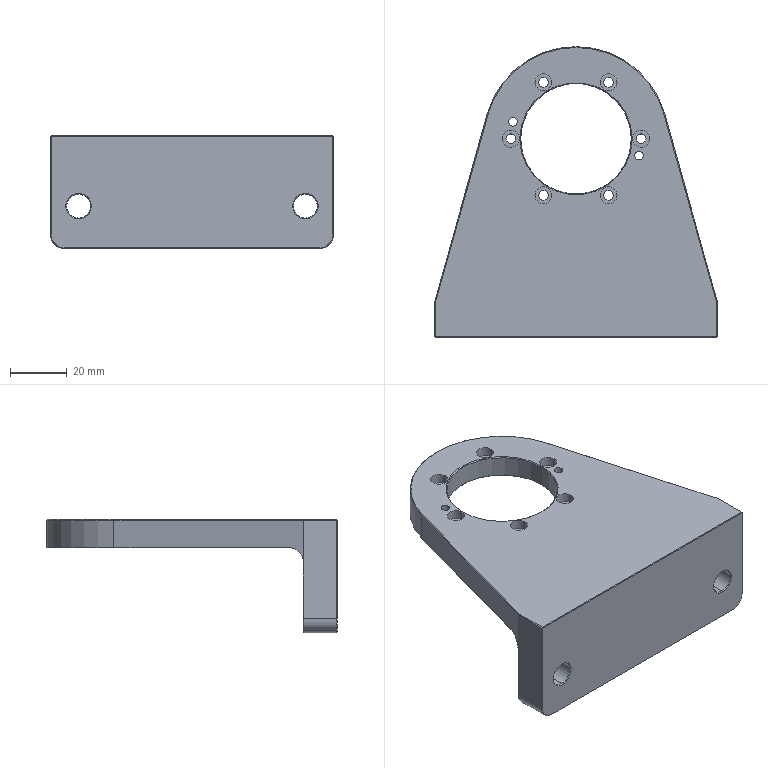NC program | NX | posted with a generic post | part box 100 x 102.5 x 40 mm
Lines 70 to 995 of 4503:
(ADAPTIVE_MILLING , TOOL : D10)
N120 T15 M6
N122 G54
N124 G17 G0 G90 X-39.298 Y62.694 B0. C0. S9500 M3
N126 G43 Z30. H15
N128 Z-17.
N130 G94 G1 Z-20. F1000.
N132 X-39.828 Y61.338 F3000.
N134 G3 X-39.298 Y60.047 R1.015
N136 X-36.138 Y59.404 R9.424
N138 X-24.642 Y59.208 R185.073
N140 G1 X-19.242 Y59.206
N142 X53.458
N144 X53.658 Y59.203
N146 X53.758 Y59.199
N148 X53.858 Y59.193
N150 X53.957 Y59.185
N152 G2 X58.292 Y56.274 R6.04
N154 X60.077 Y50.703 R13.203
N156 X60.422 Y42.315 R76.732
N158 G1 X60.429 Y40.915
N160 X60.434 Y39.015
N162 X60.437 Y35.815
N164 X60.439 Y26.715
N166 Y-52.285
N168 X60.437 Y-52.385
N170 G2 X57.938 Y-56.743 R5.754
N172 X52.455 Y-58.757 R12.082
N174 X43.972 Y-59.169 R66.869
N176 G1 X42.672 Y-59.177
N178 X40.972 Y-59.182
N180 X38.272 Y-59.186
N182 X32.672 Y-59.188
N184 X-53.528
N186 X-53.628 Y-59.187
N188 G2 X-58.106 Y-56.528 R5.815
N190 X-60.033 Y-51.012 R12.428
N192 X-60.423 Y-42.126 R73.754
N194 G1 X-60.43 Y-40.626
N196 X-60.435 Y-38.426
N198 X-60.438 Y-34.626
N200 X-60.439 Y-17.626
N202 Y38.974
N204 X-60.442 Y39.974
N206 G2 X-60.42 Y52.773 R766.33
N208 X-57.54 Y57.022 R6.066
N210 X-52.074 Y58.811 R13.054
N212 X-43.887 Y59.171 R72.631
N214 X-38.005 Y58.794 R42.391
N216 G3 X-25.915 Y58.424 R142.287
N218 G1 X-23.615 Y58.419
N220 X-20.015 Y58.415
N222 X-10.015 Y58.414
N224 X50.785
N226 X50.985 Y58.41
N228 X51.185 Y58.402
N230 G2 X57.273 Y54.557 R7.641
N232 X59.221 Y48.304 R15.498
N234 X59.615 Y38.417 R90.294
N236 G1 X59.621 Y36.817
N238 X59.626 Y34.517
N240 X59.629 Y30.617
N242 X59.63 Y15.917
N244 Y-49.483
N246 X59.628 Y-49.683
N248 G2 X55.908 Y-55.943 R7.565
N250 X49.776 Y-57.938 R15.014
N252 X40.191 Y-58.361 R82.486
N254 G1 X38.691 Y-58.369
N256 X36.691 Y-58.374
N258 X33.491 Y-58.378
N260 X26.091 Y-58.38
N262 X-50.709
N264 X-50.909 Y-58.378
N266 G2 X-57.18 Y-54.677 R7.557
N268 X-59.212 Y-48.35 R15.239
N270 X-59.609 Y-39.264 R82.815
N272 G1 X-59.617 Y-37.864
N274 X-59.623 Y-35.964
N276 X-59.627 Y-33.264
N278 X-59.63 Y-27.964
N280 Y36.236
N282 X-59.636 Y37.436
N284 G2 X-59.615 Y50.235 R604.146
N286 X-55.617 Y56.128 R7.75
N288 X-49.138 Y58.02 R16.241
N290 X-38.357 Y58.002 R55.026
N292 G3 X-21.565 Y57.627 R248.66
N294 G1 X-17.565 Y57.624
N296 X-6.765 Y57.623
N298 X48.135 Y57.622
N300 X48.435 Y57.62
N302 X48.635 Y57.618
N304 X48.835 Y57.613
N306 G2 X56.511 Y52.825 R8.831
N308 X58.428 Y46.037 R18.036
N310 X58.808 Y35.049 R112.657
N312 G1 X58.814 Y33.049
N314 X58.819 Y30.149
N316 X58.821 Y24.649
N318 X58.822 Y-20.951
N320 X58.825 Y-21.951
N322 X58.827 Y-23.551
N324 X58.826 Y-25.051
N326 X58.828 Y-25.951
N328 Y-26.851
N330 X58.83 Y-27.951
N332 X58.829 Y-28.951
N334 X58.83 Y-29.851
N336 X58.829 Y-30.851
N338 X58.831 Y-31.751
N340 X58.829 Y-32.651
N342 X58.831 Y-33.651
N344 X58.829 Y-34.751
N346 X58.831 Y-35.751
N348 X58.829 Y-36.851
N350 X58.83 Y-37.651
N352 X58.829 Y-38.651
N354 X58.831 Y-39.651
N356 X58.829 Y-40.651
N358 G2 X58.786 Y-48.25 R212.358
N360 X53.982 Y-55.292 R8.813
N362 X47.187 Y-57.185 R18.173
N364 X35.898 Y-57.56 R117.998
N366 G1 X33.898 Y-57.565
N368 X30.798 Y-57.569
N370 X24.198 Y-57.571
N372 X-48.402
N374 X-48.602 Y-57.569
N376 X-48.802 Y-57.565
N378 G2 X-56.545 Y-52.727 R8.81
N380 X-58.454 Y-45.732 R18.397
N382 X-58.811 Y-34.242 R126.498
N384 G1 X-58.817 Y-31.942
N386 X-58.82 Y-28.242
N388 X-58.821 Y-18.442
N390 X-58.822 Y33.458
N392 X-58.828 Y34.758
N394 X-58.83 Y36.258
N396 G2 X-58.807 Y48.157 R460.428
N398 X-54.076 Y55.248 R8.808
N400 X-47.192 Y57.185 R17.971
N402 X-39.101 Y57.212 R49.816
N404 G3 X-21.208 Y56.838 R325.602
N406 G1 X-17.808 Y56.834
N408 X-11.308 Y56.832
N410 X45.492 Y56.831
N412 X46.192 Y56.827
N414 X46.492 Y56.824
N416 X46.692 Y56.82
N418 G2 X55.822 Y51.112 R9.789
N420 X57.619 Y44.18 R20.375
N422 X57.999 Y32.69 R124.75
N424 G1 X58.005 Y30.69
N426 X58.01 Y27.79
N428 X58.012 Y22.49
N430 X58.013 Y-18.21
N432 X58.018 Y-19.31
N434 X58.02 Y-20.81
N436 Y-22.41
N438 X58.023 Y-23.31
N440 X58.024 Y-24.61
N442 X58.027 Y-25.51
N444 X58.026 Y-26.81
N446 X58.028 Y-27.61
N448 Y-28.81
N450 X58.029 Y-29.71
N452 X58.028 Y-30.61
N454 X58.03 Y-31.51
N456 X58.029 Y-32.51
N458 X58.031 Y-33.51
N460 X58.029 Y-34.61
N462 X58.03 Y-35.61
N464 X58.029 Y-36.41
N466 X58.031 Y-37.41
N468 X58.029 Y-38.51
N470 G2 X57.965 Y-46.608 R162.791
N472 X52.621 Y-54.424 R9.634
N474 X45.424 Y-56.366 R19.82
N476 X34.635 Y-56.745 R117.504
N478 G1 X32.835 Y-56.753
N480 X30.435 Y-56.758
N482 X26.835 Y-56.761
N484 X16.835 Y-56.762
N486 X-46.365
N488 X-46.565 Y-56.761
N490 G2 X-53.076 Y-54.646 R10.034
N492 G1 X-53.461 Y-54.486
N494 X-53.58 Y-54.418
N496 G2 X-55.736 Y-52.211 R7.144
N498 X-57.708 Y-43.572 R25.584
N500 X-58.005 Y-30.979 R182.312
N502 G1 X-58.009 Y-28.179
N504 X-58.012 Y-23.179
N506 X-58.013 Y11.221
N508 Y30.721
N510 X-58.017 Y31.621
N512 X-58.019 Y32.621
N514 G2 X-58.015 Y46.121 R784.268
N516 X-55.877 Y51.873 R9.634
N518 G1 X-55.736 Y52.211
N520 X-55.668 Y52.33
N522 G2 X-53.461 Y54.486 R7.144
N524 X-43.717 Y56.433 R24.504
N526 X-32.621 Y56.164 R346.097
N528 G3 X-12.522 Y56.041 R869.916
N530 G1 X8.478 Y56.04
N532 X42.778
N534 X43.978 Y56.033
N536 X44.478 Y56.029
N538 X44.978 Y56.02
N540 X45.178 Y56.015
N542 G2 X52.192 Y53.546 R10.616
N544 X56.022 Y46.996 R13.055
N546 X57.066 Y38.578 R38.218
N548 X57.203 Y22.18 R583.22
N550 G1 X57.204 Y7.78
N552 X57.205 Y-15.52
N554 X57.209 Y-16.42
N556 X57.211 Y-17.62
N558 X57.215 Y-18.42
N560 Y-18.92
N562 X57.214 Y-19.82
N564 X57.219 Y-20.92
N566 Y-22.02
N568 X57.222 Y-23.02
N570 Y-24.22
N572 X57.225 Y-25.22
N574 X57.224 Y-26.22
N576 X57.227 Y-27.22
N578 X57.226 Y-28.42
N580 X57.228 Y-29.32
N582 X57.227 Y-30.62
N584 X57.229 Y-31.42
N586 X57.228 Y-32.42
N588 X57.23 Y-33.52
N590 X57.229 Y-34.32
N592 X57.231 Y-35.42
N594 X57.229 Y-36.32
N596 G2 X57.165 Y-44.919 R201.547
N598 X51.289 Y-53.601 R10.297
N600 X43.784 Y-55.555 R21.276
N602 X31.795 Y-55.94 R134.94
N604 G1 X29.695 Y-55.946
N606 X26.695 Y-55.951
N608 X21.195 Y-55.953
N610 X-44.305 Y-55.954
N612 X-44.705 Y-55.952
N614 X-45.005 Y-55.948
N616 G2 X-49.614 Y-55.155 R14.255
N618 X-52.346 Y-54.948 R11.744
N620 G1 X-53.086 Y-54.642
N622 X-53.337 Y-54.539
N624 X-53.58 Y-54.418
N626 G2 X-55.736 Y-52.211 R7.227
N628 G1 X-56.198 Y-51.096
N630 G2 X-56.516 Y-47.77 R31.1
N632 X-57.185 Y-32.292 R148.725
N634 G1 X-57.192 Y-30.492
N636 X-57.199 Y-27.992
N638 X-57.202 Y-24.292
N640 X-57.204 Y-15.992
N642 X-57.205 Y28.008
N644 X-57.209 Y28.908
N646 G2 X-57.199 Y44.608 R764.429
N648 X-56.408 Y48.411 R13.691
N650 X-56.198 Y51.096 R11.906
N652 G1 X-55.854 Y51.928
N654 G3 X-57.97 Y52.356 R-1.1
N656 G1 X-58.6 Y-49.559
N658 G3 X-57.505 Y-50.664 R1.1
N660 X-56.4 Y-49.566 R1.1
N662 G1 Y48.534
N664 G2 X-56.198 Y51.096 R10.617
N666 X-54.564 Y53.663 R6.015
N668 G1 X-53.58 Y54.418
N670 X-53.461 Y54.486
N672 X-52.346 Y54.948
N674 G2 X-49.418 Y55.227 R22.217
N676 X-38.63 Y55.519 R79.437
N678 G3 X-10.533 Y55.249 R913.498
N680 G1 X16.567
N682 X40.067 Y55.248
N684 X41.867 Y55.237
N686 X42.667 Y55.232
N688 X43.167 Y55.225
N690 G2 X49.086 Y54.007 R13.093
N692 X54.523 Y47.721 R11.639
N694 X56.075 Y40.107 R26.204
N696 X56.387 Y26.913 R190.336
N698 G1 X56.392 Y24.013
N700 X56.395 Y19.113
N702 X56.396 Y-2.987
N704 Y-12.787
N706 X56.4 Y-13.687
N708 X56.402 Y-14.987
N710 X56.407 Y-15.987
N712 X56.408 Y-17.387
N714 X56.413 Y-18.487
N716 Y-19.587
N718 X56.417 Y-20.687
N720 Y-21.687
N722 X56.421 Y-22.787
N724 Y-23.887
N726 X56.424 Y-24.887
N728 X56.423 Y-26.087
N730 X56.426 Y-27.087
N732 X56.425 Y-28.187
N734 X56.428 Y-29.187
N736 X56.426 Y-30.287
N738 X56.428 Y-31.187
N740 Y-32.487
N742 G2 X56.36 Y-43.385 R285.575
N744 X49.959 Y-52.819 R10.87
N746 X42.437 Y-54.727 R22.416
N748 X30.249 Y-55.13 R135.397
N750 G1 X28.349 Y-55.136
N752 X25.649 Y-55.141
N754 X21.149 Y-55.144
N756 X6.249 Y-55.145
N758 X-39.182
N760 X-39.232 Y-55.149
N762 X-39.268 Y-55.15
N764 X-49.668
N766 G3 X-50.592 Y-55.767 R1.01
N768 G1 X-51.385 Y-57.603 Z-19.9
N770 G2 X-51.778 Y-58.218 R1.418
N772 X-52.85 Y-58.332 R1.011
N774 G1 X-53.966 Y-57.774
N776 X-55.058 Y-57.168
N778 G2 X-56.726 Y-55.945 R10.968
N780 X-57.789 Y-54.689 R7.418
N782 X-58.716 Y-53.097 R9.68
N784 X-59.266 Y-50.733 R6.939
N786 X-59.511 Y-43.244 R172.458
N788 G1 X-60.256 Y43.234
N790 G2 X-59.232 Y51.387 R31.064
N792 G1 X-58.921 Y52.574
N794 X-58.592 Y53.757
N796 G2 X-56.392 Y56.398 R4.86
N798 G1 X-54.613 Y57.4
N800 G2 X-53.424 Y57.246 R1.009
N802 G1 X-51.939 Y55.907 Z-20.
N804 X-51.27 Y55.317
N806 G3 X-50.716 Y55.15 R1.05
N808 G1 X-39.268
N810 X-39.232 Y55.149
N812 G2 X-36.033 Y54.791 R234.525
N814 G3 X-21.739 Y54.475 R237.987
N816 G1 X-19.239 Y54.467
N818 X-15.939 Y54.462
N820 X-10.939 Y54.458
N822 X2.561 Y54.457
N824 X37.361
N826 X39.061 Y54.447
N828 G2 X44.65 Y54.202 R39.414
N830 X53.145 Y47.774 R11.258
N832 X55.146 Y39.968 R22.992
N834 X55.565 Y28.48 R125.908
N836 G1 X55.573 Y26.78
N838 X55.579 Y24.68
N840 X55.584 Y21.38
N842 X55.586 Y15.68
N844 X55.587 Y7.68
N846 X55.594 Y7.581
N848 X55.597 Y7.557
N850 X55.805 Y6.657
N852 X55.815 Y6.605
N854 X56.29 Y2.855
N856 X56.294 Y2.801
N858 X56.386 Y-0.992
N860 X56.385 Y-1.025
N862 G2 X55.821 Y-6.734 R65.3
N864 G3 X55.619 Y-15.629 R121.735
N866 G1 Y-17.829
N868 X55.622 Y-20.029
N870 X55.623 Y-20.529
N872 X55.621 Y-21.329
N874 X55.622 Y-21.929
N876 X55.623 Y-22.529
N878 X55.622 Y-23.529
N880 X55.625 Y-24.729
N882 X55.623 Y-25.829
N884 X55.626 Y-26.829
N886 X55.625 Y-27.829
N888 X55.627 Y-28.929
N890 X55.626 Y-29.929
N892 X55.628 Y-30.929
N894 X55.627 Y-32.029
N896 G2 X55.549 Y-42.028 R228.856
N898 X48.958 Y-51.907 R11.314
N900 X41.251 Y-53.892 R22.815
N902 X29.863 Y-54.313 R124.104
N904 G1 X28.263 Y-54.322
N906 X26.163 Y-54.328
N908 X23.263 Y-54.333
N910 X18.163 Y-54.336
N912 X-4.937 Y-54.337
N914 X-35.537
N916 G2 X-38.514 Y-55.095 R179.175
N918 G1 X-38.585 Y-55.104
N920 X-39.183 Y-55.145
N922 G3 X-39.181 Y-57.141 R1.
N924 G1 X-38.933 Y-57.157
N926 X-36.938 Y-57.289 Z-19.9
N928 X-35.286 Y-57.395
N930 X37.839
N932 G3 X44.014 Y-56.718 R28.808
N934 G1 X45.354 Y-56.418
N936 X46.682 Y-56.07
N938 G3 X52.578 Y-53.178 R19.723
N940 X54.882 Y-51.398 R24.071
N942 X56.148 Y-49.792 R7.044
N944 X57.478 Y-47.115 R26.695
N946 X58.16 Y-44.598 R12.677
N948 X58.554 Y-40.889 R22.015
N950 G1 X59.159 Y-8.626
N952 X59.139 Y-8.427
N954 X59.088 Y-8.234
N956 X58.358 Y-6.418
N958 X58.099 Y-5.764 Z-19.935
N960 X57.824 Y-5.117 Z-19.97
N962 G3 X57.394 Y-4.721 Z-20. R1.049
N964 X55.977 Y-5.444 R1.003
N966 X55.089 Y-10.498 R100.777
N968 X54.84 Y-18.691 R94.439
N970 G1 X54.832 Y-21.191
N972 X54.827 Y-23.691
N974 X54.826 Y-26.191
N976 X54.829 Y-28.691
N978 X54.83 Y-29.291
N980 X54.828 Y-29.991
N982 X54.829 Y-30.791
N984 X54.83 Y-31.391
N986 X54.829 Y-32.291
N988 X54.83 Y-33.091
N990 X54.829 Y-33.891
N992 X54.83 Y-34.891
N994 G2 X54.662 Y-41.585 R71.054
N996 X47.791 Y-51.102 R11.67
N998 X40.075 Y-53.06 R23.64
N1000 X28.588 Y-53.502 R121.257
N1002 G1 X26.988 Y-53.511
N1004 X24.888 Y-53.518
N1006 X22.088 Y-53.524
N1008 X17.588 Y-53.527
N1010 X4.788 Y-53.528
N1012 X-32.612
N1014 X-32.712 Y-53.533
N1016 X-32.819 Y-53.547
N1018 X-35.804 Y-54.383
N1020 G3 X-35.987 Y-56.237 R1.001
N1022 X-35.33 Y-56.365 Z-19.966 R1.675
N1024 G1 X-34.009 Y-56.47 Z-19.9
N1026 X-31.907 Y-56.633
N1028 X33.093
N1030 G3 X41.798 Y-55.96 R59.876
N1032 X48.961 Y-53.908 R26.424
N1034 X53.588 Y-50.782 R18.657
N1036 X55.048 Y-49.258 R11.046
N1038 X56.633 Y-46.172 R11.229
N1040 X57.627 Y-41.314 R16.524
N1042 G1 X57.787 Y-38.823
N1044 X57.892 Y-36.329
N1046 X58.58 Y-11.806
N1048 X58.559 Y-11.593
N1050 X58.501 Y-11.388
N1052 X57.739 Y-9.591
N1054 X57.481 Y-8.972 Z-19.934
N1056 X57.203 Y-8.363 Z-19.967
N1058 G3 X56.697 Y-7.958 Z-20. R1.041
N1060 X55.398 Y-8.624 R1.004
N1062 X54.378 Y-12.795 R25.967
N1064 X54.055 Y-20.985 R80.133
N1066 G1 X54.047 Y-22.385
N1068 X54.041 Y-24.085
N1070 X54.039 Y-26.085
N1072 X54.038 Y-26.685
N1074 X54.034 Y-27.485
N1076 Y-28.285
N1078 X54.035 Y-28.885
N1080 X54.032 Y-29.785
N1082 Y-30.585
N1084 Y-31.085
N1086 X54.031 Y-31.885
N1088 X54.032 Y-32.885
N1090 X54.027 Y-34.285
N1092 Y-34.985
N1094 X54.024 Y-35.785
N1096 X54.015 Y-36.885
N1098 G2 X53.363 Y-42.828 R21.168
N1100 X46.799 Y-50.231 R11.995
N1102 X38.891 Y-52.243 R24.374
N1104 X26.904 Y-52.694 R127.347
N1106 G1 X25.204 Y-52.703
N1108 X23.004 Y-52.71
N1110 X20.004 Y-52.715
N1112 X15.004 Y-52.718
N1114 X-1.696 Y-52.72
N1116 X-29.696
N1118 X-29.796 Y-52.722
N1120 X-29.895 Y-52.732
N1122 X-29.934 Y-52.738
N1124 X-32.823 Y-53.548
N1126 G3 X-33.006 Y-55.402 R1.001
N1128 X-32.349 Y-55.53 Z-19.966 R1.675
N1130 G1 X-31.028 Y-55.635 Z-19.9
N1132 X-28.926 Y-55.798
N1134 X34.199
N1136 G3 X41.014 Y-55.127 R35.788
N1138 X47.599 Y-53.244 R34.595
N1140 X51.331 Y-51.033 R15.261
N1142 G1 X52.025 Y-50.413
N1144 X52.68 Y-49.751
N1146 X53.481 Y-48.876
N1148 X54.269 Y-47.989
N1150 G3 X55.694 Y-45.397 R8.933
N1152 G1 X55.921 Y-44.688
N1154 X56.109 Y-43.967
N1156 G3 X56.8 Y-40.293 R39.084
N1158 G1 X56.925 Y-39.055
N1160 X57.002 Y-37.812
N1162 X57.864 Y-14.306
N1164 X57.844 Y-14.088
N1166 X57.785 Y-13.878
N1168 X57.025 Y-12.092
N1170 X56.766 Y-11.472 Z-19.934
N1172 X56.487 Y-10.862 Z-19.967
N1174 G3 X55.983 Y-10.459 Z-20. R1.041
N1176 X54.682 Y-11.124 R1.004
N1178 G2 X53.929 Y-13.453 R66.85
N1180 G3 X53.325 Y-19.713 R31.007
N1182 X53.201 Y-36.512 R978.881
N1184 G2 X52.221 Y-42.701 R17.893
N1186 X45.342 Y-49.589 R12.517
N1188 X37.294 Y-51.469 R26.261
N1190 X25.305 Y-51.886 R141.796
N1192 G1 X23.505 Y-51.895
N1194 X21.205 Y-51.902
N1196 X18.005 Y-51.907
N1198 X12.805 Y-51.91
N1200 X-6.895 Y-51.911
N1202 X-26.795
N1204 X-26.895 Y-51.912
N1206 X-26.994 Y-51.921
N1208 X-27.05 Y-51.93
N1210 X-29.938 Y-52.74
N1212 G3 X-30.122 Y-54.594 R1.001
N1214 X-29.465 Y-54.722 Z-19.966 R1.675
N1216 G1 X-28.144 Y-54.826 Z-19.9
N1218 X-26.041 Y-54.99
N1220 X32.709
N1222 G3 X40.136 Y-54.254 R38.314
N1224 G1 X42.705 Y-53.726
N1226 G3 X49.38 Y-50.748 R20.14
N1228 X51.755 Y-48.931 R19.855
N1230 X53.42 Y-46.918 R11.577
N1232 X55.442 Y-42.423 R13.539
N1234 X55.947 Y-39.358 R19.463
N1236 G1 X56.173 Y-36.872
N1238 X56.341 Y-34.381
N1240 X57.315 Y-15.966
N1242 X57.296 Y-15.729
N1244 X57.227 Y-15.5
N1246 X56.447 Y-13.781
N1248 X56.18 Y-13.18 Z-19.933
N1250 X55.89 Y-12.589 Z-19.966
N1252 G3 X55.349 Y-12.193 Z-20. R1.039
N1254 X54.133 Y-12.784 R1.005
N1256 X52.661 Y-19.172 R16.325
N1258 X52.44 Y-31.868 R253.297
N1260 G2 X52.188 Y-38.46 R59.193
N1262 X44.786 Y-48.548 R12.545
N1264 X36.78 Y-50.585 R25.095
N1266 X25.195 Y-51.068 R117.402
N1268 G1 X23.695 Y-51.079
N1270 X21.895 Y-51.087
N1272 X19.595 Y-51.094
N1274 X16.395 Y-51.098
N1276 X10.895 Y-51.101
N1278 X-11.005 Y-51.102
N1280 X-23.905
N1282 X-24.005 Y-51.103
N1284 X-24.105 Y-51.112
N1286 X-24.164 Y-51.122
N1288 X-27.053 Y-51.931
N1290 G3 X-27.236 Y-53.786 R1.001
N1292 X-26.579 Y-53.913 Z-19.966 R1.674
N1294 G1 X-25.258 Y-54.018 Z-19.9
N1296 X-23.156 Y-54.181
N1298 X30.594
N1300 G3 X38.043 Y-53.565 R45.87
N1302 G1 X39.707 Y-53.289
N1304 X41.362 Y-52.967
N1306 G3 X46.284 Y-51.224 R21.017
N1308 G1 X47.391 Y-50.613
N1310 X48.487 Y-49.982
N1312 G3 X51.373 Y-47.508 R13.567
N1314 X53.98 Y-43.3 R12.588
N1316 X55.129 Y-38.48 R16.719
N1318 G1 X55.376 Y-35.996
N1320 X55.573 Y-33.507
N1322 X56.617 Y-17.733
N1324 X56.6 Y-17.488
N1326 X56.529 Y-17.252
N1328 X55.751 Y-15.547
N1330 X55.483 Y-14.945 Z-19.933
N1332 X55.192 Y-14.355 Z-19.966
N1334 G3 X54.651 Y-13.96 Z-20. R1.039
N1336 X53.436 Y-14.551 R1.005
N1338 X52.516 Y-16.82 R49.659
N1340 X51.801 Y-22.563 R25.85
N1342 X51.596 Y-34.461 R772.828
N1344 G2 X50.476 Y-40.928 R18.353
N1346 X43.483 Y-47.859 R12.987
N1348 X35.149 Y-49.829 R27.118
N1350 X22.961 Y-50.266 R142.214
N1352 G1 X21.461 Y-50.274
N1354 X19.361 Y-50.282
N1356 X16.561 Y-50.288
N1358 X12.361 Y-50.292
N1360 X3.361 Y-50.294
N1362 X-21.039
N1364 X-21.139 Y-50.296
N1366 X-21.238 Y-50.307
N1368 X-21.275 Y-50.313
N1370 X-24.164 Y-51.122
N1372 G3 X-24.347 Y-52.976 R1.001
N1374 X-23.69 Y-53.104 Z-19.966 R1.674
N1376 G1 X-22.369 Y-53.209 Z-19.9
N1378 X-20.267 Y-53.372
N1380 X29.108
N1382 G3 X37.788 Y-52.589 R48.938
N1384 G1 X40.86 Y-52.018
N1386 G3 X44.369 Y-50.793 R17.143
N1388 X47.662 Y-49.018 R22.672
N1390 X50.515 Y-46.618 R18.947
N1392 X52.597 Y-43.833 R17.2
N1394 X53.637 Y-41.306 R12.099
N1396 X54.539 Y-35.779 R23.838
N1398 G1 X55.115 Y-19.782
N1400 X55.007 Y-18.621
N1402 X54.88 Y-17.463
N1404 X54.81 Y-16.773 Z-19.935
N1406 X54.722 Y-16.084 Z-19.969
N1408 G3 X54.4 Y-15.576 Z-20. R1.046
N1410 X52.865 Y-15.884 R1.003
N1412 X51.251 Y-21.092 R11.886
N1414 X50.876 Y-30.18 R102.783
N1416 G2 X50.514 Y-36.765 R51.24
N1418 X42.716 Y-46.936 R13.032
N1420 X34.302 Y-48.989 R26.84
N1422 X21.215 Y-49.46 R143.887
N1424 G1 X19.315 Y-49.469
N1426 X16.915 Y-49.476
N1428 X13.615 Y-49.481
N1430 X8.215 Y-49.484
N1432 X-9.885 Y-49.485
N1434 X-18.185
N1436 G3 X-21.276 Y-50.313 R31.257
N1438 X-21.459 Y-52.167 R1.001
N1440 X-20.802 Y-52.295 Z-19.966 R1.674
N1442 G1 X-19.481 Y-52.4 Z-19.9
N1444 X-17.379 Y-52.563
N1446 X25.121
N1448 G3 X35.083 Y-51.948 R82.023
N1450 G1 X38.8 Y-51.475
N1452 G3 X42.499 Y-50.404 R16.766
N1454 X45.202 Y-49.119 R27.7
N1456 G1 X46.218 Y-48.566
N1458 X47.208 Y-47.969
N1460 G3 X49.666 Y-45.807 R13.519
N1462 X52.253 Y-41.592 R11.977
N1464 X53.538 Y-36.474 R22.892
N1466 G1 X53.695 Y-35.081
N1468 X53.799 Y-33.683
N1470 X54.432 Y-21.117
N1472 X54.427 Y-20.961
N1474 X54.197 Y-18.799
N1476 X54.127 Y-18.108 Z-19.935
N1478 X54.039 Y-17.419 Z-19.97
N1480 G3 X53.717 Y-16.911 Z-20. R1.047
N1482 X52.182 Y-17.22 R1.003
N1484 X50.479 Y-22.608 R12.457
N1486 X50.072 Y-30.895 R104.762
N1488 G2 X49.406 Y-37.247 R29.345
N1490 X42.148 Y-45.925 R13.109
N1492 X33.971 Y-48.096 R25.482
N1494 X22.589 Y-48.63 R109.277
N1496 G1 X21.389 Y-48.641
N1498 X19.789 Y-48.652
N1500 X17.789 Y-48.661
N1502 X15.289 Y-48.668
N1504 X11.789 Y-48.673
N1506 X5.889 Y-48.676
N1508 X-15.311 Y-48.677
N1510 X-15.41 Y-48.683
N1512 X-15.509 Y-48.697
N1514 X-18.398 Y-49.507
N1516 G3 X-18.582 Y-51.361 R1.001
N1518 X-17.924 Y-51.489 Z-19.966 R1.674
N1520 G1 X-16.604 Y-51.593 Z-19.9
N1522 X-14.501 Y-51.757
N1524 X27.999
N1526 G3 X35.438 Y-51.086 R42.087
N1528 G1 X38.017 Y-50.604
N1530 G3 X45.549 Y-47.419 R21.783
N1532 X48.255 Y-45.417 R32.285
N1534 X50.414 Y-42.708 R10.137
N1536 X51.85 Y-39.535 R28.839
N1538 X52.661 Y-35.919 R15.2
N1540 X53.373 Y-27.205 R244.774
N1542 G1 X53.659 Y-22.542
N1544 X53.402 Y-20.287
N1546 X53.33 Y-19.62 Z-19.934
N1548 X53.235 Y-18.956 Z-19.967
N1550 G3 X52.866 Y-18.426 Z-20. R1.041
N1552 X51.407 Y-18.734 R1.004
N1554 X49.848 Y-22.959 R9.202
N1556 X49.298 Y-30.535 R72.328
N1558 G2 X48.414 Y-36.956 R25.749
N1560 X41.028 Y-45.184 R13.394
N1562 X32.733 Y-47.307 R26.42
N1564 X19.95 Y-47.833 R129.027
N1566 G1 X18.35 Y-47.844
N1568 X16.45 Y-47.852
N1570 X13.95 Y-47.859
N1572 X10.45 Y-47.864
N1574 X4.55 Y-47.867
N1576 X-12.45 Y-47.868
N1578 X-15.51 Y-48.698
N1580 G3 X-15.694 Y-50.552 R1.001
N1582 X-15.036 Y-50.68 Z-19.966 R1.674
N1584 G1 X-13.716 Y-50.784 Z-19.9
N1586 X-11.613 Y-50.948
N1588 X24.012
N1590 G3 X34.851 Y-50.134 R76.515
N1592 X40.034 Y-48.88 R31.722
N1594 G1 X41.116 Y-48.519
N1596 X42.181 Y-48.113
N1598 G3 X45.261 Y-46.282 R14.646
N1600 X48.631 Y-43.143 R23.448
N1602 X50.623 Y-39.714 R11.691
N1604 X51.855 Y-34.906 R19.635
N1606 G1 X52.19 Y-32.431
N1608 X52.477 Y-29.951
N1610 X53.151 Y-23.318
N1612 X52.877 Y-21.107
N1614 X52.798 Y-20.445 Z-19.933
N1616 X52.695 Y-19.786 Z-19.967
N1618 G3 X52.312 Y-19.256 Z-20. R1.04
N1620 X50.896 Y-19.535 R1.004
N1622 X49.075 Y-24.239 R9.87
N1624 X48.475 Y-31.01 R88.508
N1626 G2 X46.971 Y-37.705 R19.322
N1628 X39.619 Y-44.579 R13.909
N1630 X31.081 Y-46.56 R28.682
N1632 X17.994 Y-47.03 R149.44
N1634 G1 X16.294 Y-47.039
N1636 X14.094 Y-47.047
N1638 X11.194 Y-47.053
N1640 X6.894 Y-47.057
N1642 X-1.906 Y-47.059
N1644 X-9.506
N1646 X-9.606 Y-47.063
N1648 X-9.706 Y-47.074
N1650 X-9.729 Y-47.078
N1652 X-12.714 Y-47.914
N1654 G3 X-12.897 Y-49.768 R1.001
N1656 X-12.24 Y-49.896 Z-19.966 R1.673
N1658 G1 X-10.92 Y-50.001 Z-19.9
N1660 X-8.817 Y-50.164
N1662 X24.308
N1664 G3 X32.999 Y-49.445 R53.484
N1666 G1 X36.201 Y-48.898
N1668 G3 X43.757 Y-45.782 R21.206
N1670 X46.469 Y-43.788 R31.774
N1672 X48.663 Y-41.102 R10.628
N1674 X50.892 Y-35.25 R20.017
N1676 G1 X51.16 Y-33.873
N1678 X51.379 Y-32.489
N1680 X52.445 Y-24.527
N1682 Y-24.266
N1684 X52.178 Y-22.2
N1686 X52.097 Y-21.538 Z-19.933
N1688 X51.993 Y-20.879 Z-19.967
N1690 G3 X51.61 Y-20.35 Z-20. R1.04
N1692 X50.195 Y-20.63 R1.004
N1694 X48.307 Y-25.415 R10.128
N1696 X47.579 Y-31.671 R227.85
N1698 G2 X44.93 Y-38.919 R15.56
N1700 X37.287 Y-44.3 R15.299
N1702 X28.054 Y-45.919 R36.588
N1704 X11.46 Y-46.242 R284.625
N1706 G1 X7.96 Y-46.247
N1708 X2.06 Y-46.25
N1710 X-6.64 Y-46.251
N1712 X-6.74 Y-46.256
N1714 X-6.842 Y-46.269
N1716 X-9.73 Y-47.078
N1718 G3 X-9.914 Y-48.933 R1.001
N1720 X-9.257 Y-49.061 Z-19.966 R1.673
N1722 G1 X-7.936 Y-49.165 Z-19.9
N1724 X-5.833 Y-49.328
N1726 X24.792
N1728 G3 X33.457 Y-48.47 R44.556
N1730 X37.27 Y-47.577 R37.998
N1732 X41.712 Y-45.818 R30.523
N1734 X45.202 Y-43.293 R13.758
N1736 G1 X45.997 Y-42.5
N1738 X46.761 Y-41.676
N1740 G3 X48.84 Y-38.288 R14.156
N1742 X50.176 Y-34.153 R16.998
N1744 G1 X51.689 Y-25.706
N1746 X51.7 Y-25.547
N1748 X51.694 Y-25.388
N1750 X51.407 Y-23.384
N1752 X51.318 Y-22.731 Z-19.933
N1754 X51.205 Y-22.081 Z-19.966
N1756 G3 X50.8 Y-21.551 Z-20. R1.039
N1758 X49.439 Y-21.809 R1.005
N1760 X47.722 Y-25.534 R7.808
N1762 X46.783 Y-31.357 R150.673
N1764 G2 X43.289 Y-39.089 R15.247
N1766 X35.597 Y-43.73 R16.529
N1768 X26.226 Y-45.157 R40.906
N1770 X10.931 Y-45.431 R302.9
N1772 G1 X7.631 Y-45.437
N1774 X2.431 Y-45.441
N1776 X-3.769 Y-45.442
N1778 X-3.869 Y-45.448
N1780 X-3.968 Y-45.464
N1782 X-6.857 Y-46.273
N1784 G3 X-7.04 Y-48.127 R1.001
N1786 X-6.383 Y-48.255 Z-19.966 R1.673
N1788 G1 X-5.062 Y-48.36 Z-19.9
N1790 X-2.96 Y-48.523
N1792 X23.29
N1794 G3 X30.739 Y-47.907 R45.87
N1796 X34.9 Y-47.079 R44.214
N1798 X38.807 Y-45.757 R25.52
N1800 X41.308 Y-44.422 R20.947
N1802 X44.422 Y-42.346 R43.628
N1804 X47.524 Y-38.518 R10.31
N1806 X49.075 Y-34.457 R21.84
N1808 G1 X50.145 Y-30.423
N1810 X51.164 Y-26.376
N1812 X51.188 Y-26.178
N1814 X51.18 Y-25.979
N1816 X50.87 Y-24.068
N1818 X50.77 Y-23.418 Z-19.933
N1820 X50.646 Y-22.772 Z-19.966
N1822 G3 X50.227 Y-22.248 Z-20. R1.039
N1824 X48.914 Y-22.479 R1.005
N1826 X46.932 Y-26.568 R8.547
N1828 G2 X45.751 Y-32.04 R159.611
N1830 X36.648 Y-42.223 R14.77
N1832 X27.689 Y-44.164 R31.441
N1834 X15.1 Y-44.599 R156.854
N1836 G1 X13.3 Y-44.61
N1838 X11.2 Y-44.619
N1840 X8.5 Y-44.625
N1842 X4.6 Y-44.63
N1844 X-0.9 Y-44.633
N1846 X-0.999 Y-44.641
N1848 X-1.072 Y-44.653
N1850 X-4.057 Y-45.489
N1852 G3 X-4.241 Y-47.343 R1.001
N1854 X-3.583 Y-47.471 Z-19.966 R1.673
N1856 G1 X-2.263 Y-47.576 Z-19.9
N1858 X-0.16 Y-47.739
N1860 X21.09
N1862 G3 X31.01 Y-46.844 R55.916
N1864 G1 X33.745 Y-46.332
N1866 G3 X39.386 Y-44.426 R26.5
N1868 X43.799 Y-41.28 R16.518
N1870 G1 X44.627 Y-40.454
N1872 X45.418 Y-39.592
N1874 G3 X47.18 Y-36.7 R12.614
N1876 X48.275 Y-33.919 R28.103
N1878 G1 X50.484 Y-27.24
N1880 X50.528 Y-27.
N1882 X50.52 Y-26.755
N1884 X50.201 Y-24.918
N1886 X50.093 Y-24.269 Z-19.933
N1888 X49.961 Y-23.625 Z-19.966
N1890 G3 X49.536 Y-23.105 Z-20. R1.039
N1892 X48.234 Y-23.343 R1.005
N1894 X46.123 Y-27.486 R9.287
N1896 G2 X44.408 Y-33.125 R44.108
N1898 X35.771 Y-41.405 R15.182
N1900 X26.811 Y-43.345 R32.042
N1902 X14.023 Y-43.791 R158.949
N1904 G1 X12.223 Y-43.801
N1906 X10.023 Y-43.81
N1908 X7.223 Y-43.817
N1910 X3.323 Y-43.821
N1912 X2.023 Y-43.822
N1914 X1.923 Y-43.828
N1916 X1.824 Y-43.841
N1918 X-1.161 Y-44.678
N1920 G3 X-1.345 Y-46.532 R1.001
N1922 X-0.688 Y-46.66 Z-19.966 R1.672
N1924 G1 X0.633 Y-46.764 Z-19.9
N1926 X2.736 Y-46.928
N1928 X18.986
N1930 G3 X28.928 Y-46.167 R65.951
N1932 G1 X32.218 Y-45.649
N1934 G3 X37.989 Y-43.959 R28.873
N1936 X43.03 Y-40.384 R15.858
N1938 G1 X43.885 Y-39.487
N1940 X44.702 Y-38.556
N1942 G3 X46.506 Y-35.78 R16.864
N1944 X47.795 Y-32.997 R29.389
N1946 G1 X49.68 Y-28.262
N1948 G3 X49.734 Y-27.711 R1.056
N1950 G1 X49.406 Y-25.927
N1952 X49.292 Y-25.28 Z-19.933
N1954 X49.154 Y-24.637 Z-19.966
N1956 G3 X48.723 Y-24.122 Z-20. R1.039
N1958 X47.43 Y-24.364 R1.005
N1960 X45.395 Y-27.938 R8.896
N1962 G2 X43.207 Y-33.409 R35.496
N1964 X34.265 Y-40.838 R16.016